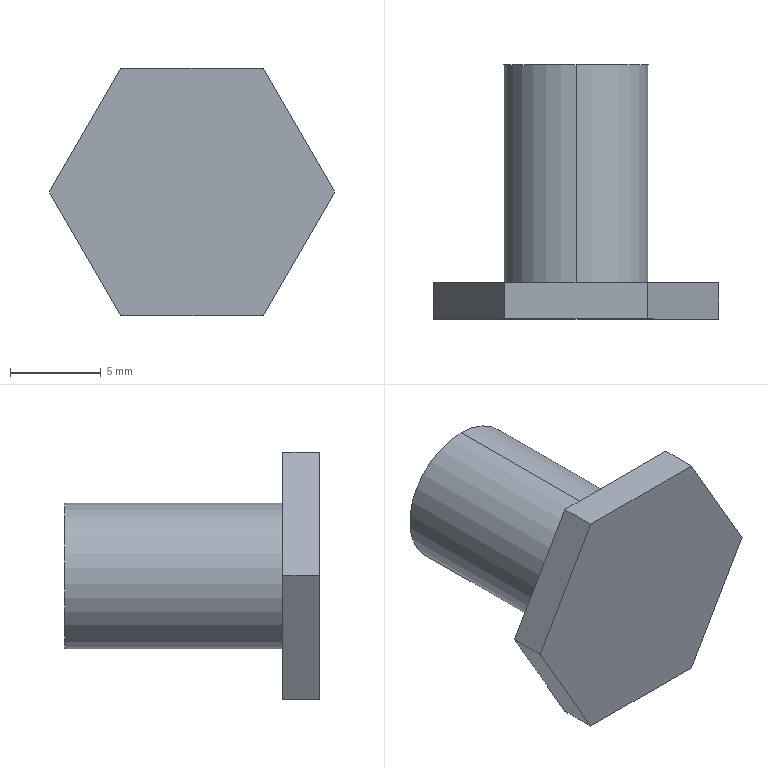Part | SolidWorks | features BaseBody 1 | 1 solid | 11 faces | box 15.704 x 14 x 13.6 mm | volume 923.546 mm3 | plane 9 | cylinder 2 | commonest cylinder face diameters 8 x2
STEP:
#1=CARTESIAN_POINT('',(0.,14.,-4.));
#2=VERTEX_POINT('',#1);
#3=CARTESIAN_POINT('',(0.,14.,4.));
#4=VERTEX_POINT('',#3);
#5=CARTESIAN_POINT('',(0.,14.,0.));
#6=DIRECTION('',(0.,-1.,0.));
#7=DIRECTION('',(0.,0.,-1.));
#8=AXIS2_PLACEMENT_3D('',#5,#6,#7);
#9=CIRCLE('',#8,4.);
#10=EDGE_CURVE('',#2,#4,#9,.T.);
#11=ORIENTED_EDGE('',*,*,#10,.T.);
#12=CARTESIAN_POINT('',(0.,2.,4.));
#13=VERTEX_POINT('',#12);
#14=CARTESIAN_POINT('',(0.,14.,4.));
#15=DIRECTION('',(0.,-1.,0.));
#16=VECTOR('',#15,1000.);
#17=LINE('',#14,#16);
#18=EDGE_CURVE('',#4,#13,#17,.T.);
#19=ORIENTED_EDGE('',*,*,#18,.T.);
#20=CARTESIAN_POINT('',(0.,2.,-4.));
#21=VERTEX_POINT('',#20);
#22=CARTESIAN_POINT('',(0.,2.,0.));
#23=DIRECTION('',(0.,-1.,0.));
#24=DIRECTION('',(0.,0.,-1.));
#25=AXIS2_PLACEMENT_3D('',#22,#23,#24);
#26=CIRCLE('',#25,4.);
#27=EDGE_CURVE('',#21,#13,#26,.T.);
#28=ORIENTED_EDGE('',*,*,#27,.F.);
#29=CARTESIAN_POINT('',(0.,14.,-4.));
#30=DIRECTION('',(0.,-1.,0.));
#31=VECTOR('',#30,1000.);
#32=LINE('',#29,#31);
#33=EDGE_CURVE('',#2,#21,#32,.T.);
#34=ORIENTED_EDGE('',*,*,#33,.F.);
#35=EDGE_LOOP('',(#11,#19,#28,#34));
#36=FACE_OUTER_BOUND('',#35,.T.);
#37=CARTESIAN_POINT('',(0.,14.,0.));
#38=DIRECTION('',(0.,-1.,0.));
#39=DIRECTION('',(0.,0.,-1.));
#40=AXIS2_PLACEMENT_3D('',#37,#38,#39);
#41=CYLINDRICAL_SURFACE('',#40,4.);
#42=ADVANCED_FACE('',(#36),#41,.T.);
#43=CARTESIAN_POINT('',(-3.926,0.,6.8));
#44=VERTEX_POINT('',#43);
#45=CARTESIAN_POINT('',(3.926,0.,6.8));
#46=VERTEX_POINT('',#45);
#47=CARTESIAN_POINT('',(0.,0.,6.8));
#48=DIRECTION('',(1.,0.,0.));
#49=VECTOR('',#48,1000.);
#50=LINE('',#47,#49);
#51=EDGE_CURVE('',#44,#46,#50,.T.);
#52=ORIENTED_EDGE('',*,*,#51,.F.);
#53=CARTESIAN_POINT('',(-7.852,0.,0.));
#54=VERTEX_POINT('',#53);
#55=CARTESIAN_POINT('',(-7.852,0.,0.));
#56=DIRECTION('',(0.5,0.,0.866));
#57=VECTOR('',#56,1000.);
#58=LINE('',#55,#57);
#59=EDGE_CURVE('',#54,#44,#58,.T.);
#60=ORIENTED_EDGE('',*,*,#59,.F.);
#61=CARTESIAN_POINT('',(-3.926,0.,-6.8));
#62=VERTEX_POINT('',#61);
#63=CARTESIAN_POINT('',(-3.926,0.,-6.8));
#64=DIRECTION('',(-0.5,0.,0.866));
#65=VECTOR('',#64,1000.);
#66=LINE('',#63,#65);
#67=EDGE_CURVE('',#62,#54,#66,.T.);
#68=ORIENTED_EDGE('',*,*,#67,.F.);
#69=CARTESIAN_POINT('',(3.926,0.,-6.8));
#70=VERTEX_POINT('',#69);
#71=CARTESIAN_POINT('',(0.,0.,-6.8));
#72=DIRECTION('',(-1.,0.,0.));
#73=VECTOR('',#72,1000.);
#74=LINE('',#71,#73);
#75=EDGE_CURVE('',#70,#62,#74,.T.);
#76=ORIENTED_EDGE('',*,*,#75,.F.);
#77=CARTESIAN_POINT('',(7.852,0.,0.));
#78=VERTEX_POINT('',#77);
#79=CARTESIAN_POINT('',(7.852,0.,0.));
#80=DIRECTION('',(-0.5,0.,-0.866));
#81=VECTOR('',#80,1000.);
#82=LINE('',#79,#81);
#83=EDGE_CURVE('',#78,#70,#82,.T.);
#84=ORIENTED_EDGE('',*,*,#83,.F.);
#85=CARTESIAN_POINT('',(3.926,0.,6.8));
#86=DIRECTION('',(0.5,0.,-0.866));
#87=VECTOR('',#86,1000.);
#88=LINE('',#85,#87);
#89=EDGE_CURVE('',#46,#78,#88,.T.);
#90=ORIENTED_EDGE('',*,*,#89,.F.);
#91=EDGE_LOOP('',(#52,#60,#68,#76,#84,#90));
#92=FACE_OUTER_BOUND('',#91,.T.);
#93=CARTESIAN_POINT('',(0.,0.,0.));
#94=DIRECTION('',(0.,1.,0.));
#95=DIRECTION('',(0.,0.,1.));
#96=AXIS2_PLACEMENT_3D('',#93,#94,#95);
#97=PLANE('',#96);
#98=ADVANCED_FACE('',(#92),#97,.F.);
#99=CARTESIAN_POINT('',(7.852,2.,0.));
#100=VERTEX_POINT('',#99);
#101=CARTESIAN_POINT('',(7.852,2.,0.));
#102=DIRECTION('',(0.,-1.,0.));
#103=VECTOR('',#102,1000.);
#104=LINE('',#101,#103);
#105=EDGE_CURVE('',#100,#78,#104,.T.);
#106=ORIENTED_EDGE('',*,*,#105,.F.);
#107=CARTESIAN_POINT('',(3.926,2.,6.8));
#108=VERTEX_POINT('',#107);
#109=CARTESIAN_POINT('',(3.926,2.,6.8));
#110=DIRECTION('',(0.5,0.,-0.866));
#111=VECTOR('',#110,1000.);
#112=LINE('',#109,#111);
#113=EDGE_CURVE('',#108,#100,#112,.T.);
#114=ORIENTED_EDGE('',*,*,#113,.F.);
#115=CARTESIAN_POINT('',(3.926,2.,6.8));
#116=DIRECTION('',(0.,1.,0.));
#117=VECTOR('',#116,1000.);
#118=LINE('',#115,#117);
#119=EDGE_CURVE('',#46,#108,#118,.T.);
#120=ORIENTED_EDGE('',*,*,#119,.F.);
#121=ORIENTED_EDGE('',*,*,#89,.T.);
#122=EDGE_LOOP('',(#106,#114,#120,#121));
#123=FACE_OUTER_BOUND('',#122,.T.);
#124=CARTESIAN_POINT('',(3.926,2.,6.8));
#125=DIRECTION('',(-0.866,0.,-0.5));
#126=DIRECTION('',(-0.5,0.,0.866));
#127=AXIS2_PLACEMENT_3D('',#124,#125,#126);
#128=PLANE('',#127);
#129=ADVANCED_FACE('',(#123),#128,.F.);
#130=ORIENTED_EDGE('',*,*,#119,.T.);
#131=CARTESIAN_POINT('',(-3.926,2.,6.8));
#132=VERTEX_POINT('',#131);
#133=CARTESIAN_POINT('',(-3.926,2.,6.8));
#134=DIRECTION('',(1.,0.,0.));
#135=VECTOR('',#134,1000.);
#136=LINE('',#133,#135);
#137=EDGE_CURVE('',#132,#108,#136,.T.);
#138=ORIENTED_EDGE('',*,*,#137,.F.);
#139=CARTESIAN_POINT('',(-3.926,2.,6.8));
#140=DIRECTION('',(0.,1.,0.));
#141=VECTOR('',#140,1000.);
#142=LINE('',#139,#141);
#143=EDGE_CURVE('',#44,#132,#142,.T.);
#144=ORIENTED_EDGE('',*,*,#143,.F.);
#145=ORIENTED_EDGE('',*,*,#51,.T.);
#146=EDGE_LOOP('',(#130,#138,#144,#145));
#147=FACE_OUTER_BOUND('',#146,.T.);
#148=CARTESIAN_POINT('',(-3.926,2.,6.8));
#149=DIRECTION('',(0.,0.,-1.));
#150=DIRECTION('',(-1.,0.,0.));
#151=AXIS2_PLACEMENT_3D('',#148,#149,#150);
#152=PLANE('',#151);
#153=ADVANCED_FACE('',(#147),#152,.F.);
#154=ORIENTED_EDGE('',*,*,#143,.T.);
#155=CARTESIAN_POINT('',(-7.852,2.,0.));
#156=VERTEX_POINT('',#155);
#157=CARTESIAN_POINT('',(-7.852,2.,0.));
#158=DIRECTION('',(0.5,0.,0.866));
#159=VECTOR('',#158,1000.);
#160=LINE('',#157,#159);
#161=EDGE_CURVE('',#156,#132,#160,.T.);
#162=ORIENTED_EDGE('',*,*,#161,.F.);
#163=CARTESIAN_POINT('',(-7.852,2.,0.));
#164=DIRECTION('',(0.,1.,0.));
#165=VECTOR('',#164,1000.);
#166=LINE('',#163,#165);
#167=EDGE_CURVE('',#54,#156,#166,.T.);
#168=ORIENTED_EDGE('',*,*,#167,.F.);
#169=ORIENTED_EDGE('',*,*,#59,.T.);
#170=EDGE_LOOP('',(#154,#162,#168,#169));
#171=FACE_OUTER_BOUND('',#170,.T.);
#172=CARTESIAN_POINT('',(-7.852,2.,0.));
#173=DIRECTION('',(0.866,0.,-0.5));
#174=DIRECTION('',(-0.5,0.,-0.866));
#175=AXIS2_PLACEMENT_3D('',#172,#173,#174);
#176=PLANE('',#175);
#177=ADVANCED_FACE('',(#171),#176,.F.);
#178=ORIENTED_EDGE('',*,*,#167,.T.);
#179=CARTESIAN_POINT('',(-3.926,2.,-6.8));
#180=VERTEX_POINT('',#179);
#181=CARTESIAN_POINT('',(-3.926,2.,-6.8));
#182=DIRECTION('',(-0.5,0.,0.866));
#183=VECTOR('',#182,1000.);
#184=LINE('',#181,#183);
#185=EDGE_CURVE('',#180,#156,#184,.T.);
#186=ORIENTED_EDGE('',*,*,#185,.F.);
#187=CARTESIAN_POINT('',(-3.926,2.,-6.8));
#188=DIRECTION('',(0.,1.,0.));
#189=VECTOR('',#188,1000.);
#190=LINE('',#187,#189);
#191=EDGE_CURVE('',#62,#180,#190,.T.);
#192=ORIENTED_EDGE('',*,*,#191,.F.);
#193=ORIENTED_EDGE('',*,*,#67,.T.);
#194=EDGE_LOOP('',(#178,#186,#192,#193));
#195=FACE_OUTER_BOUND('',#194,.T.);
#196=CARTESIAN_POINT('',(-3.926,2.,-6.8));
#197=DIRECTION('',(0.866,0.,0.5));
#198=DIRECTION('',(0.5,0.,-0.866));
#199=AXIS2_PLACEMENT_3D('',#196,#197,#198);
#200=PLANE('',#199);
#201=ADVANCED_FACE('',(#195),#200,.F.);
#202=ORIENTED_EDGE('',*,*,#191,.T.);
#203=CARTESIAN_POINT('',(3.926,2.,-6.8));
#204=VERTEX_POINT('',#203);
#205=CARTESIAN_POINT('',(3.926,2.,-6.8));
#206=DIRECTION('',(-1.,0.,0.));
#207=VECTOR('',#206,1000.);
#208=LINE('',#205,#207);
#209=EDGE_CURVE('',#204,#180,#208,.T.);
#210=ORIENTED_EDGE('',*,*,#209,.F.);
#211=CARTESIAN_POINT('',(3.926,2.,-6.8));
#212=DIRECTION('',(0.,1.,0.));
#213=VECTOR('',#212,1000.);
#214=LINE('',#211,#213);
#215=EDGE_CURVE('',#70,#204,#214,.T.);
#216=ORIENTED_EDGE('',*,*,#215,.F.);
#217=ORIENTED_EDGE('',*,*,#75,.T.);
#218=EDGE_LOOP('',(#202,#210,#216,#217));
#219=FACE_OUTER_BOUND('',#218,.T.);
#220=CARTESIAN_POINT('',(3.926,2.,-6.8));
#221=DIRECTION('',(0.,0.,1.));
#222=DIRECTION('',(1.,0.,0.));
#223=AXIS2_PLACEMENT_3D('',#220,#221,#222);
#224=PLANE('',#223);
#225=ADVANCED_FACE('',(#219),#224,.F.);
#226=ORIENTED_EDGE('',*,*,#215,.T.);
#227=CARTESIAN_POINT('',(7.852,2.,0.));
#228=DIRECTION('',(-0.5,0.,-0.866));
#229=VECTOR('',#228,1000.);
#230=LINE('',#227,#229);
#231=EDGE_CURVE('',#100,#204,#230,.T.);
#232=ORIENTED_EDGE('',*,*,#231,.F.);
#233=ORIENTED_EDGE('',*,*,#105,.T.);
#234=ORIENTED_EDGE('',*,*,#83,.T.);
#235=EDGE_LOOP('',(#226,#232,#233,#234));
#236=FACE_OUTER_BOUND('',#235,.T.);
#237=CARTESIAN_POINT('',(7.852,2.,0.));
#238=DIRECTION('',(-0.866,0.,0.5));
#239=DIRECTION('',(0.5,0.,0.866));
#240=AXIS2_PLACEMENT_3D('',#237,#238,#239);
#241=PLANE('',#240);
#242=ADVANCED_FACE('',(#236),#241,.F.);
#243=ORIENTED_EDGE('',*,*,#161,.T.);
#244=ORIENTED_EDGE('',*,*,#137,.T.);
#245=ORIENTED_EDGE('',*,*,#113,.T.);
#246=ORIENTED_EDGE('',*,*,#231,.T.);
#247=ORIENTED_EDGE('',*,*,#209,.T.);
#248=ORIENTED_EDGE('',*,*,#185,.T.);
#249=EDGE_LOOP('',(#243,#244,#245,#246,#247,#248));
#250=FACE_OUTER_BOUND('',#249,.T.);
#251=ORIENTED_EDGE('',*,*,#27,.T.);
#252=CARTESIAN_POINT('',(0.,2.,0.));
#253=DIRECTION('',(0.,-1.,0.));
#254=DIRECTION('',(0.,0.,-1.));
#255=AXIS2_PLACEMENT_3D('',#252,#253,#254);
#256=CIRCLE('',#255,4.);
#257=EDGE_CURVE('',#13,#21,#256,.T.);
#258=ORIENTED_EDGE('',*,*,#257,.T.);
#259=EDGE_LOOP('',(#251,#258));
#260=FACE_BOUND('',#259,.T.);
#261=CARTESIAN_POINT('',(0.,2.,0.));
#262=DIRECTION('',(0.,1.,0.));
#263=DIRECTION('',(0.,0.,1.));
#264=AXIS2_PLACEMENT_3D('',#261,#262,#263);
#265=PLANE('',#264);
#266=ADVANCED_FACE('',(#250,#260),#265,.T.);
#267=ORIENTED_EDGE('',*,*,#18,.F.);
#268=CARTESIAN_POINT('',(0.,14.,0.));
#269=DIRECTION('',(0.,-1.,0.));
#270=DIRECTION('',(0.,0.,-1.));
#271=AXIS2_PLACEMENT_3D('',#268,#269,#270);
#272=CIRCLE('',#271,4.);
#273=EDGE_CURVE('',#4,#2,#272,.T.);
#274=ORIENTED_EDGE('',*,*,#273,.T.);
#275=ORIENTED_EDGE('',*,*,#33,.T.);
#276=ORIENTED_EDGE('',*,*,#257,.F.);
#277=EDGE_LOOP('',(#267,#274,#275,#276));
#278=FACE_OUTER_BOUND('',#277,.T.);
#279=CARTESIAN_POINT('',(0.,14.,0.));
#280=DIRECTION('',(0.,-1.,0.));
#281=DIRECTION('',(0.,0.,-1.));
#282=AXIS2_PLACEMENT_3D('',#279,#280,#281);
#283=CYLINDRICAL_SURFACE('',#282,4.);
#284=ADVANCED_FACE('',(#278),#283,.T.);
#285=ORIENTED_EDGE('',*,*,#10,.F.);
#286=ORIENTED_EDGE('',*,*,#273,.F.);
#287=EDGE_LOOP('',(#285,#286));
#288=FACE_OUTER_BOUND('',#287,.T.);
#289=CARTESIAN_POINT('',(0.,14.,0.));
#290=DIRECTION('',(0.,1.,0.));
#291=DIRECTION('',(0.,0.,1.));
#292=AXIS2_PLACEMENT_3D('',#289,#290,#291);
#293=PLANE('',#292);
#294=ADVANCED_FACE('',(#288),#293,.T.);
#295=CLOSED_SHELL('',(#42,#98,#129,#153,#177,#201,#225,#242,#266,#284,#294));
#296=MANIFOLD_SOLID_BREP('',#295);
#297=CARTESIAN_POINT('',(0.,0.,0.));
#298=DIRECTION('',(0.,0.,1.));
#299=DIRECTION('',(1.,0.,0.));
#300=AXIS2_PLACEMENT_3D('',#297,#298,#299);
#301=(LENGTH_UNIT()NAMED_UNIT(*)SI_UNIT(.MILLI.,.METRE.));
#302=UNCERTAINTY_MEASURE_WITH_UNIT(LENGTH_MEASURE(0.00001),#301,'','');
#303=(NAMED_UNIT(*)PLANE_ANGLE_UNIT()SI_UNIT($,.RADIAN.));
#304=(NAMED_UNIT(*)SI_UNIT($,.STERADIAN.)SOLID_ANGLE_UNIT());
#305=(GEOMETRIC_REPRESENTATION_CONTEXT(3)GLOBAL_UNCERTAINTY_ASSIGNED_CONTEXT((#302))GLOBAL_UNIT_ASSIGNED_CONTEXT((#301,#303,#304))REPRESENTATION_CONTEXT('',''));
#306=ADVANCED_BREP_SHAPE_REPRESENTATION('',(#296,#300),#305);